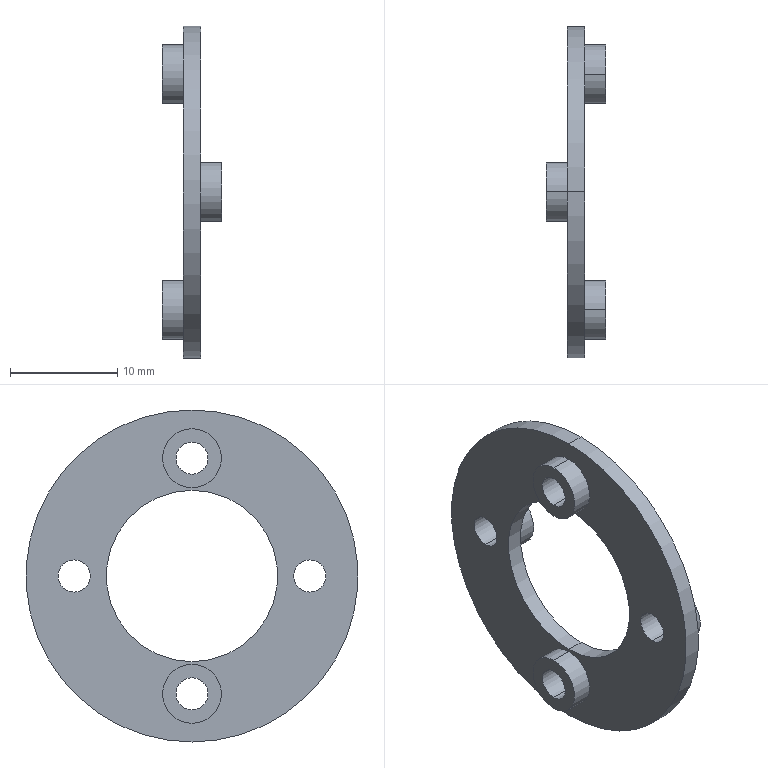Part | SolidWorks | features BaseBody 1 | 1 solid | 26 faces | box 5.6 x 31 x 31 mm | volume 974.208 mm3 | cylinder 20 | plane 6 | commonest cylinder face diameters 3 x8 5.5 x8 16 x2 31 x2
STEP:
#1=CARTESIAN_POINT('',(0.,0.,15.5));
#2=VERTEX_POINT('',#1);
#3=CARTESIAN_POINT('',(0.,0.,-15.5));
#4=VERTEX_POINT('',#3);
#5=CARTESIAN_POINT('',(0.,0.,0.));
#6=DIRECTION('',(1.,0.,0.));
#7=DIRECTION('',(0.,0.,-1.));
#8=AXIS2_PLACEMENT_3D('',#5,#6,#7);
#9=CIRCLE('',#8,15.5);
#10=EDGE_CURVE('',#2,#4,#9,.T.);
#11=ORIENTED_EDGE('',*,*,#10,.T.);
#12=CARTESIAN_POINT('',(1.6,0.,-15.5));
#13=VERTEX_POINT('',#12);
#14=CARTESIAN_POINT('',(1.6,0.,-15.5));
#15=DIRECTION('',(1.,0.,0.));
#16=VECTOR('',#15,1000.);
#17=LINE('',#14,#16);
#18=EDGE_CURVE('',#4,#13,#17,.T.);
#19=ORIENTED_EDGE('',*,*,#18,.T.);
#20=CARTESIAN_POINT('',(1.6,0.,15.5));
#21=VERTEX_POINT('',#20);
#22=CARTESIAN_POINT('',(1.6,0.,0.));
#23=DIRECTION('',(1.,0.,0.));
#24=DIRECTION('',(0.,0.,-1.));
#25=AXIS2_PLACEMENT_3D('',#22,#23,#24);
#26=CIRCLE('',#25,15.5);
#27=EDGE_CURVE('',#21,#13,#26,.T.);
#28=ORIENTED_EDGE('',*,*,#27,.F.);
#29=CARTESIAN_POINT('',(1.6,0.,15.5));
#30=DIRECTION('',(1.,0.,0.));
#31=VECTOR('',#30,1000.);
#32=LINE('',#29,#31);
#33=EDGE_CURVE('',#2,#21,#32,.T.);
#34=ORIENTED_EDGE('',*,*,#33,.F.);
#35=EDGE_LOOP('',(#11,#19,#28,#34));
#36=FACE_OUTER_BOUND('',#35,.T.);
#37=CARTESIAN_POINT('',(1.6,0.,0.));
#38=DIRECTION('',(1.,0.,0.));
#39=DIRECTION('',(0.,0.,1.));
#40=AXIS2_PLACEMENT_3D('',#37,#38,#39);
#41=CYLINDRICAL_SURFACE('',#40,15.5);
#42=ADVANCED_FACE('',(#36),#41,.T.);
#43=CARTESIAN_POINT('',(0.,0.,-8.));
#44=VERTEX_POINT('',#43);
#45=CARTESIAN_POINT('',(0.,0.,8.));
#46=VERTEX_POINT('',#45);
#47=CARTESIAN_POINT('',(0.,0.,0.));
#48=DIRECTION('',(1.,0.,0.));
#49=DIRECTION('',(0.,0.,-1.));
#50=AXIS2_PLACEMENT_3D('',#47,#48,#49);
#51=CIRCLE('',#50,8.);
#52=EDGE_CURVE('',#44,#46,#51,.T.);
#53=ORIENTED_EDGE('',*,*,#52,.F.);
#54=CARTESIAN_POINT('',(1.6,0.,-8.));
#55=VERTEX_POINT('',#54);
#56=CARTESIAN_POINT('',(1.6,0.,-8.));
#57=DIRECTION('',(1.,0.,0.));
#58=VECTOR('',#57,1000.);
#59=LINE('',#56,#58);
#60=EDGE_CURVE('',#44,#55,#59,.T.);
#61=ORIENTED_EDGE('',*,*,#60,.T.);
#62=CARTESIAN_POINT('',(1.6,0.,8.));
#63=VERTEX_POINT('',#62);
#64=CARTESIAN_POINT('',(1.6,0.,0.));
#65=DIRECTION('',(1.,0.,0.));
#66=DIRECTION('',(0.,0.,-1.));
#67=AXIS2_PLACEMENT_3D('',#64,#65,#66);
#68=CIRCLE('',#67,8.);
#69=EDGE_CURVE('',#55,#63,#68,.T.);
#70=ORIENTED_EDGE('',*,*,#69,.T.);
#71=CARTESIAN_POINT('',(1.6,0.,8.));
#72=DIRECTION('',(1.,0.,0.));
#73=VECTOR('',#72,1000.);
#74=LINE('',#71,#73);
#75=EDGE_CURVE('',#46,#63,#74,.T.);
#76=ORIENTED_EDGE('',*,*,#75,.F.);
#77=EDGE_LOOP('',(#53,#61,#70,#76));
#78=FACE_OUTER_BOUND('',#77,.T.);
#79=CARTESIAN_POINT('',(1.6,0.,0.));
#80=DIRECTION('',(1.,0.,0.));
#81=DIRECTION('',(0.,0.,1.));
#82=AXIS2_PLACEMENT_3D('',#79,#80,#81);
#83=CYLINDRICAL_SURFACE('',#82,8.);
#84=ADVANCED_FACE('',(#78),#83,.F.);
#85=CARTESIAN_POINT('',(0.,11.,1.5));
#86=VERTEX_POINT('',#85);
#87=CARTESIAN_POINT('',(0.,11.,-1.5));
#88=VERTEX_POINT('',#87);
#89=CARTESIAN_POINT('',(0.,11.,0.));
#90=DIRECTION('',(-1.,0.,0.));
#91=DIRECTION('',(0.,0.,-1.));
#92=AXIS2_PLACEMENT_3D('',#89,#90,#91);
#93=CIRCLE('',#92,1.5);
#94=EDGE_CURVE('',#86,#88,#93,.T.);
#95=ORIENTED_EDGE('',*,*,#94,.T.);
#96=CARTESIAN_POINT('',(3.6,11.,-1.5));
#97=VERTEX_POINT('',#96);
#98=CARTESIAN_POINT('',(1.6,11.,-1.5));
#99=DIRECTION('',(1.,0.,0.));
#100=VECTOR('',#99,1000.);
#101=LINE('',#98,#100);
#102=EDGE_CURVE('',#88,#97,#101,.T.);
#103=ORIENTED_EDGE('',*,*,#102,.T.);
#104=CARTESIAN_POINT('',(3.6,11.,1.5));
#105=VERTEX_POINT('',#104);
#106=CARTESIAN_POINT('',(3.6,11.,0.));
#107=DIRECTION('',(-1.,0.,0.));
#108=DIRECTION('',(0.,0.,1.));
#109=AXIS2_PLACEMENT_3D('',#106,#107,#108);
#110=CIRCLE('',#109,1.5);
#111=EDGE_CURVE('',#105,#97,#110,.T.);
#112=ORIENTED_EDGE('',*,*,#111,.F.);
#113=CARTESIAN_POINT('',(1.6,11.,1.5));
#114=DIRECTION('',(1.,0.,0.));
#115=VECTOR('',#114,1000.);
#116=LINE('',#113,#115);
#117=EDGE_CURVE('',#86,#105,#116,.T.);
#118=ORIENTED_EDGE('',*,*,#117,.F.);
#119=EDGE_LOOP('',(#95,#103,#112,#118));
#120=FACE_OUTER_BOUND('',#119,.T.);
#121=CARTESIAN_POINT('',(1.6,11.,0.));
#122=DIRECTION('',(1.,0.,0.));
#123=DIRECTION('',(0.,0.,1.));
#124=AXIS2_PLACEMENT_3D('',#121,#122,#123);
#125=CYLINDRICAL_SURFACE('',#124,1.5);
#126=ADVANCED_FACE('',(#120),#125,.F.);
#127=CARTESIAN_POINT('',(-2.,0.,12.5));
#128=VERTEX_POINT('',#127);
#129=CARTESIAN_POINT('',(-2.,0.,9.5));
#130=VERTEX_POINT('',#129);
#131=CARTESIAN_POINT('',(-2.,0.,11.));
#132=DIRECTION('',(-1.,0.,0.));
#133=DIRECTION('',(0.,0.,1.));
#134=AXIS2_PLACEMENT_3D('',#131,#132,#133);
#135=CIRCLE('',#134,1.5);
#136=EDGE_CURVE('',#128,#130,#135,.T.);
#137=ORIENTED_EDGE('',*,*,#136,.T.);
#138=CARTESIAN_POINT('',(1.6,0.,9.5));
#139=VERTEX_POINT('',#138);
#140=CARTESIAN_POINT('',(1.6,0.,9.5));
#141=DIRECTION('',(1.,0.,0.));
#142=VECTOR('',#141,1000.);
#143=LINE('',#140,#142);
#144=EDGE_CURVE('',#130,#139,#143,.T.);
#145=ORIENTED_EDGE('',*,*,#144,.T.);
#146=CARTESIAN_POINT('',(1.6,0.,12.5));
#147=VERTEX_POINT('',#146);
#148=CARTESIAN_POINT('',(1.6,0.,11.));
#149=DIRECTION('',(1.,0.,0.));
#150=DIRECTION('',(0.,0.,-1.));
#151=AXIS2_PLACEMENT_3D('',#148,#149,#150);
#152=CIRCLE('',#151,1.5);
#153=EDGE_CURVE('',#139,#147,#152,.T.);
#154=ORIENTED_EDGE('',*,*,#153,.T.);
#155=CARTESIAN_POINT('',(1.6,0.,12.5));
#156=DIRECTION('',(1.,0.,0.));
#157=VECTOR('',#156,1000.);
#158=LINE('',#155,#157);
#159=EDGE_CURVE('',#128,#147,#158,.T.);
#160=ORIENTED_EDGE('',*,*,#159,.F.);
#161=EDGE_LOOP('',(#137,#145,#154,#160));
#162=FACE_OUTER_BOUND('',#161,.T.);
#163=CARTESIAN_POINT('',(1.6,0.,11.));
#164=DIRECTION('',(1.,0.,0.));
#165=DIRECTION('',(0.,0.,1.));
#166=AXIS2_PLACEMENT_3D('',#163,#164,#165);
#167=CYLINDRICAL_SURFACE('',#166,1.5);
#168=ADVANCED_FACE('',(#162),#167,.F.);
#169=CARTESIAN_POINT('',(0.,-11.,1.5));
#170=VERTEX_POINT('',#169);
#171=CARTESIAN_POINT('',(0.,-11.,-1.5));
#172=VERTEX_POINT('',#171);
#173=CARTESIAN_POINT('',(0.,-11.,0.));
#174=DIRECTION('',(-1.,0.,0.));
#175=DIRECTION('',(0.,0.,-1.));
#176=AXIS2_PLACEMENT_3D('',#173,#174,#175);
#177=CIRCLE('',#176,1.5);
#178=EDGE_CURVE('',#170,#172,#177,.T.);
#179=ORIENTED_EDGE('',*,*,#178,.T.);
#180=CARTESIAN_POINT('',(3.6,-11.,-1.5));
#181=VERTEX_POINT('',#180);
#182=CARTESIAN_POINT('',(1.6,-11.,-1.5));
#183=DIRECTION('',(1.,0.,0.));
#184=VECTOR('',#183,1000.);
#185=LINE('',#182,#184);
#186=EDGE_CURVE('',#172,#181,#185,.T.);
#187=ORIENTED_EDGE('',*,*,#186,.T.);
#188=CARTESIAN_POINT('',(3.6,-11.,1.5));
#189=VERTEX_POINT('',#188);
#190=CARTESIAN_POINT('',(3.6,-11.,0.));
#191=DIRECTION('',(-1.,0.,0.));
#192=DIRECTION('',(0.,0.,1.));
#193=AXIS2_PLACEMENT_3D('',#190,#191,#192);
#194=CIRCLE('',#193,1.5);
#195=EDGE_CURVE('',#189,#181,#194,.T.);
#196=ORIENTED_EDGE('',*,*,#195,.F.);
#197=CARTESIAN_POINT('',(1.6,-11.,1.5));
#198=DIRECTION('',(1.,0.,0.));
#199=VECTOR('',#198,1000.);
#200=LINE('',#197,#199);
#201=EDGE_CURVE('',#170,#189,#200,.T.);
#202=ORIENTED_EDGE('',*,*,#201,.F.);
#203=EDGE_LOOP('',(#179,#187,#196,#202));
#204=FACE_OUTER_BOUND('',#203,.T.);
#205=CARTESIAN_POINT('',(1.6,-11.,0.));
#206=DIRECTION('',(1.,0.,0.));
#207=DIRECTION('',(0.,0.,1.));
#208=AXIS2_PLACEMENT_3D('',#205,#206,#207);
#209=CYLINDRICAL_SURFACE('',#208,1.5);
#210=ADVANCED_FACE('',(#204),#209,.F.);
#211=CARTESIAN_POINT('',(-2.,0.,-9.5));
#212=VERTEX_POINT('',#211);
#213=CARTESIAN_POINT('',(-2.,0.,-12.5));
#214=VERTEX_POINT('',#213);
#215=CARTESIAN_POINT('',(-2.,0.,-11.));
#216=DIRECTION('',(-1.,0.,0.));
#217=DIRECTION('',(0.,0.,1.));
#218=AXIS2_PLACEMENT_3D('',#215,#216,#217);
#219=CIRCLE('',#218,1.5);
#220=EDGE_CURVE('',#212,#214,#219,.T.);
#221=ORIENTED_EDGE('',*,*,#220,.T.);
#222=CARTESIAN_POINT('',(1.6,0.,-12.5));
#223=VERTEX_POINT('',#222);
#224=CARTESIAN_POINT('',(1.6,0.,-12.5));
#225=DIRECTION('',(1.,0.,0.));
#226=VECTOR('',#225,1000.);
#227=LINE('',#224,#226);
#228=EDGE_CURVE('',#214,#223,#227,.T.);
#229=ORIENTED_EDGE('',*,*,#228,.T.);
#230=CARTESIAN_POINT('',(1.6,0.,-9.5));
#231=VERTEX_POINT('',#230);
#232=CARTESIAN_POINT('',(1.6,0.,-11.));
#233=DIRECTION('',(1.,0.,0.));
#234=DIRECTION('',(0.,0.,-1.));
#235=AXIS2_PLACEMENT_3D('',#232,#233,#234);
#236=CIRCLE('',#235,1.5);
#237=EDGE_CURVE('',#223,#231,#236,.T.);
#238=ORIENTED_EDGE('',*,*,#237,.T.);
#239=CARTESIAN_POINT('',(1.6,0.,-9.5));
#240=DIRECTION('',(1.,0.,0.));
#241=VECTOR('',#240,1000.);
#242=LINE('',#239,#241);
#243=EDGE_CURVE('',#212,#231,#242,.T.);
#244=ORIENTED_EDGE('',*,*,#243,.F.);
#245=EDGE_LOOP('',(#221,#229,#238,#244));
#246=FACE_OUTER_BOUND('',#245,.T.);
#247=CARTESIAN_POINT('',(1.6,0.,-11.));
#248=DIRECTION('',(1.,0.,0.));
#249=DIRECTION('',(0.,0.,1.));
#250=AXIS2_PLACEMENT_3D('',#247,#248,#249);
#251=CYLINDRICAL_SURFACE('',#250,1.5);
#252=ADVANCED_FACE('',(#246),#251,.F.);
#253=CARTESIAN_POINT('',(1.6,11.,2.75));
#254=VERTEX_POINT('',#253);
#255=CARTESIAN_POINT('',(1.6,11.,-2.75));
#256=VERTEX_POINT('',#255);
#257=CARTESIAN_POINT('',(1.6,11.,0.));
#258=DIRECTION('',(1.,0.,0.));
#259=DIRECTION('',(0.,0.,-1.));
#260=AXIS2_PLACEMENT_3D('',#257,#258,#259);
#261=CIRCLE('',#260,2.75);
#262=EDGE_CURVE('',#254,#256,#261,.T.);
#263=ORIENTED_EDGE('',*,*,#262,.T.);
#264=CARTESIAN_POINT('',(3.6,11.,-2.75));
#265=VERTEX_POINT('',#264);
#266=CARTESIAN_POINT('',(1.6,11.,-2.75));
#267=DIRECTION('',(1.,0.,0.));
#268=VECTOR('',#267,1000.);
#269=LINE('',#266,#268);
#270=EDGE_CURVE('',#256,#265,#269,.T.);
#271=ORIENTED_EDGE('',*,*,#270,.T.);
#272=CARTESIAN_POINT('',(3.6,11.,2.75));
#273=VERTEX_POINT('',#272);
#274=CARTESIAN_POINT('',(3.6,11.,0.));
#275=DIRECTION('',(-1.,0.,0.));
#276=DIRECTION('',(0.,0.,1.));
#277=AXIS2_PLACEMENT_3D('',#274,#275,#276);
#278=CIRCLE('',#277,2.75);
#279=EDGE_CURVE('',#265,#273,#278,.T.);
#280=ORIENTED_EDGE('',*,*,#279,.T.);
#281=CARTESIAN_POINT('',(1.6,11.,2.75));
#282=DIRECTION('',(1.,0.,0.));
#283=VECTOR('',#282,1000.);
#284=LINE('',#281,#283);
#285=EDGE_CURVE('',#254,#273,#284,.T.);
#286=ORIENTED_EDGE('',*,*,#285,.F.);
#287=EDGE_LOOP('',(#263,#271,#280,#286));
#288=FACE_OUTER_BOUND('',#287,.T.);
#289=CARTESIAN_POINT('',(1.6,11.,0.));
#290=DIRECTION('',(1.,0.,0.));
#291=DIRECTION('',(0.,0.,1.));
#292=AXIS2_PLACEMENT_3D('',#289,#290,#291);
#293=CYLINDRICAL_SURFACE('',#292,2.75);
#294=ADVANCED_FACE('',(#288),#293,.T.);
#295=CARTESIAN_POINT('',(1.6,-11.,2.75));
#296=VERTEX_POINT('',#295);
#297=CARTESIAN_POINT('',(1.6,-11.,-2.75));
#298=VERTEX_POINT('',#297);
#299=CARTESIAN_POINT('',(1.6,-11.,0.));
#300=DIRECTION('',(1.,0.,0.));
#301=DIRECTION('',(0.,0.,-1.));
#302=AXIS2_PLACEMENT_3D('',#299,#300,#301);
#303=CIRCLE('',#302,2.75);
#304=EDGE_CURVE('',#296,#298,#303,.T.);
#305=ORIENTED_EDGE('',*,*,#304,.T.);
#306=CARTESIAN_POINT('',(3.6,-11.,-2.75));
#307=VERTEX_POINT('',#306);
#308=CARTESIAN_POINT('',(1.6,-11.,-2.75));
#309=DIRECTION('',(1.,0.,0.));
#310=VECTOR('',#309,1000.);
#311=LINE('',#308,#310);
#312=EDGE_CURVE('',#298,#307,#311,.T.);
#313=ORIENTED_EDGE('',*,*,#312,.T.);
#314=CARTESIAN_POINT('',(3.6,-11.,2.75));
#315=VERTEX_POINT('',#314);
#316=CARTESIAN_POINT('',(3.6,-11.,0.));
#317=DIRECTION('',(-1.,0.,0.));
#318=DIRECTION('',(0.,0.,1.));
#319=AXIS2_PLACEMENT_3D('',#316,#317,#318);
#320=CIRCLE('',#319,2.75);
#321=EDGE_CURVE('',#307,#315,#320,.T.);
#322=ORIENTED_EDGE('',*,*,#321,.T.);
#323=CARTESIAN_POINT('',(1.6,-11.,2.75));
#324=DIRECTION('',(1.,0.,0.));
#325=VECTOR('',#324,1000.);
#326=LINE('',#323,#325);
#327=EDGE_CURVE('',#296,#315,#326,.T.);
#328=ORIENTED_EDGE('',*,*,#327,.F.);
#329=EDGE_LOOP('',(#305,#313,#322,#328));
#330=FACE_OUTER_BOUND('',#329,.T.);
#331=CARTESIAN_POINT('',(1.6,-11.,0.));
#332=DIRECTION('',(1.,0.,0.));
#333=DIRECTION('',(0.,0.,1.));
#334=AXIS2_PLACEMENT_3D('',#331,#332,#333);
#335=CYLINDRICAL_SURFACE('',#334,2.75);
#336=ADVANCED_FACE('',(#330),#335,.T.);
#337=CARTESIAN_POINT('',(-2.,0.,-13.75));
#338=VERTEX_POINT('',#337);
#339=CARTESIAN_POINT('',(-2.,0.,-8.25));
#340=VERTEX_POINT('',#339);
#341=CARTESIAN_POINT('',(-2.,0.,-11.));
#342=DIRECTION('',(-1.,0.,0.));
#343=DIRECTION('',(0.,0.,1.));
#344=AXIS2_PLACEMENT_3D('',#341,#342,#343);
#345=CIRCLE('',#344,2.75);
#346=EDGE_CURVE('',#338,#340,#345,.T.);
#347=ORIENTED_EDGE('',*,*,#346,.F.);
#348=CARTESIAN_POINT('',(0.,0.,-13.75));
#349=VERTEX_POINT('',#348);
#350=CARTESIAN_POINT('',(-2.,0.,-13.75));
#351=DIRECTION('',(1.,0.,0.));
#352=VECTOR('',#351,1000.);
#353=LINE('',#350,#352);
#354=EDGE_CURVE('',#338,#349,#353,.T.);
#355=ORIENTED_EDGE('',*,*,#354,.T.);
#356=CARTESIAN_POINT('',(0.,0.,-8.25));
#357=VERTEX_POINT('',#356);
#358=CARTESIAN_POINT('',(0.,0.,-11.));
#359=DIRECTION('',(-1.,0.,0.));
#360=DIRECTION('',(0.,0.,1.));
#361=AXIS2_PLACEMENT_3D('',#358,#359,#360);
#362=CIRCLE('',#361,2.75);
#363=EDGE_CURVE('',#349,#357,#362,.T.);
#364=ORIENTED_EDGE('',*,*,#363,.T.);
#365=CARTESIAN_POINT('',(-2.,0.,-8.25));
#366=DIRECTION('',(1.,0.,0.));
#367=VECTOR('',#366,1000.);
#368=LINE('',#365,#367);
#369=EDGE_CURVE('',#340,#357,#368,.T.);
#370=ORIENTED_EDGE('',*,*,#369,.F.);
#371=EDGE_LOOP('',(#347,#355,#364,#370));
#372=FACE_OUTER_BOUND('',#371,.T.);
#373=CARTESIAN_POINT('',(-2.,0.,-11.));
#374=DIRECTION('',(1.,0.,0.));
#375=DIRECTION('',(0.,0.,1.));
#376=AXIS2_PLACEMENT_3D('',#373,#374,#375);
#377=CYLINDRICAL_SURFACE('',#376,2.75);
#378=ADVANCED_FACE('',(#372),#377,.T.);
#379=CARTESIAN_POINT('',(-2.,0.,8.25));
#380=VERTEX_POINT('',#379);
#381=CARTESIAN_POINT('',(-2.,0.,13.75));
#382=VERTEX_POINT('',#381);
#383=CARTESIAN_POINT('',(-2.,0.,11.));
#384=DIRECTION('',(-1.,0.,0.));
#385=DIRECTION('',(0.,0.,1.));
#386=AXIS2_PLACEMENT_3D('',#383,#384,#385);
#387=CIRCLE('',#386,2.75);
#388=EDGE_CURVE('',#380,#382,#387,.T.);
#389=ORIENTED_EDGE('',*,*,#388,.F.);
#390=CARTESIAN_POINT('',(0.,0.,8.25));
#391=VERTEX_POINT('',#390);
#392=CARTESIAN_POINT('',(-2.,0.,8.25));
#393=DIRECTION('',(1.,0.,0.));
#394=VECTOR('',#393,1000.);
#395=LINE('',#392,#394);
#396=EDGE_CURVE('',#380,#391,#395,.T.);
#397=ORIENTED_EDGE('',*,*,#396,.T.);
#398=CARTESIAN_POINT('',(0.,0.,13.75));
#399=VERTEX_POINT('',#398);
#400=CARTESIAN_POINT('',(0.,0.,11.));
#401=DIRECTION('',(-1.,0.,0.));
#402=DIRECTION('',(0.,0.,1.));
#403=AXIS2_PLACEMENT_3D('',#400,#401,#402);
#404=CIRCLE('',#403,2.75);
#405=EDGE_CURVE('',#391,#399,#404,.T.);
#406=ORIENTED_EDGE('',*,*,#405,.T.);
#407=CARTESIAN_POINT('',(-2.,0.,13.75));
#408=DIRECTION('',(1.,0.,0.));
#409=VECTOR('',#408,1000.);
#410=LINE('',#407,#409);
#411=EDGE_CURVE('',#382,#399,#410,.T.);
#412=ORIENTED_EDGE('',*,*,#411,.F.);
#413=EDGE_LOOP('',(#389,#397,#406,#412));
#414=FACE_OUTER_BOUND('',#413,.T.);
#415=CARTESIAN_POINT('',(-2.,0.,11.));
#416=DIRECTION('',(1.,0.,0.));
#417=DIRECTION('',(0.,0.,1.));
#418=AXIS2_PLACEMENT_3D('',#415,#416,#417);
#419=CYLINDRICAL_SURFACE('',#418,2.75);
#420=ADVANCED_FACE('',(#414),#419,.T.);
#421=ORIENTED_EDGE('',*,*,#396,.F.);
#422=CARTESIAN_POINT('',(-2.,0.,11.));
#423=DIRECTION('',(-1.,0.,0.));
#424=DIRECTION('',(0.,0.,1.));
#425=AXIS2_PLACEMENT_3D('',#422,#423,#424);
#426=CIRCLE('',#425,2.75);
#427=EDGE_CURVE('',#382,#380,#426,.T.);
#428=ORIENTED_EDGE('',*,*,#427,.F.);
#429=ORIENTED_EDGE('',*,*,#411,.T.);
#430=CARTESIAN_POINT('',(0.,0.,11.));
#431=DIRECTION('',(-1.,0.,0.));
#432=DIRECTION('',(0.,0.,1.));
#433=AXIS2_PLACEMENT_3D('',#430,#431,#432);
#434=CIRCLE('',#433,2.75);
#435=EDGE_CURVE('',#399,#391,#434,.T.);
#436=ORIENTED_EDGE('',*,*,#435,.T.);
#437=EDGE_LOOP('',(#421,#428,#429,#436));
#438=FACE_OUTER_BOUND('',#437,.T.);
#439=CARTESIAN_POINT('',(-2.,0.,11.));
#440=DIRECTION('',(1.,0.,0.));
#441=DIRECTION('',(0.,0.,1.));
#442=AXIS2_PLACEMENT_3D('',#439,#440,#441);
#443=CYLINDRICAL_SURFACE('',#442,2.75);
#444=ADVANCED_FACE('',(#438),#443,.T.);
#445=ORIENTED_EDGE('',*,*,#136,.F.);
#446=CARTESIAN_POINT('',(-2.,0.,11.));
#447=DIRECTION('',(-1.,0.,0.));
#448=DIRECTION('',(0.,0.,1.));
#449=AXIS2_PLACEMENT_3D('',#446,#447,#448);
#450=CIRCLE('',#449,1.5);
#451=EDGE_CURVE('',#130,#128,#450,.T.);
#452=ORIENTED_EDGE('',*,*,#451,.F.);
#453=EDGE_LOOP('',(#445,#452));
#454=FACE_BOUND('',#453,.T.);
#455=ORIENTED_EDGE('',*,*,#427,.T.);
#456=ORIENTED_EDGE('',*,*,#388,.T.);
#457=EDGE_LOOP('',(#455,#456));
#458=FACE_OUTER_BOUND('',#457,.T.);
#459=CARTESIAN_POINT('',(-2.,0.,12.5));
#460=DIRECTION('',(-1.,0.,0.));
#461=DIRECTION('',(0.,0.,1.));
#462=AXIS2_PLACEMENT_3D('',#459,#460,#461);
#463=PLANE('',#462);
#464=ADVANCED_FACE('',(#454,#458),#463,.T.);
#465=ORIENTED_EDGE('',*,*,#354,.F.);
#466=CARTESIAN_POINT('',(-2.,0.,-11.));
#467=DIRECTION('',(-1.,0.,0.));
#468=DIRECTION('',(0.,0.,1.));
#469=AXIS2_PLACEMENT_3D('',#466,#467,#468);
#470=CIRCLE('',#469,2.75);
#471=EDGE_CURVE('',#340,#338,#470,.T.);
#472=ORIENTED_EDGE('',*,*,#471,.F.);
#473=ORIENTED_EDGE('',*,*,#369,.T.);
#474=CARTESIAN_POINT('',(0.,0.,-11.));
#475=DIRECTION('',(-1.,0.,0.));
#476=DIRECTION('',(0.,0.,1.));
#477=AXIS2_PLACEMENT_3D('',#474,#475,#476);
#478=CIRCLE('',#477,2.75);
#479=EDGE_CURVE('',#357,#349,#478,.T.);
#480=ORIENTED_EDGE('',*,*,#479,.T.);
#481=EDGE_LOOP('',(#465,#472,#473,#480));
#482=FACE_OUTER_BOUND('',#481,.T.);
#483=CARTESIAN_POINT('',(-2.,0.,-11.));
#484=DIRECTION('',(1.,0.,0.));
#485=DIRECTION('',(0.,0.,1.));
#486=AXIS2_PLACEMENT_3D('',#483,#484,#485);
#487=CYLINDRICAL_SURFACE('',#486,2.75);
#488=ADVANCED_FACE('',(#482),#487,.T.);
#489=ORIENTED_EDGE('',*,*,#220,.F.);
#490=CARTESIAN_POINT('',(-2.,0.,-11.));
#491=DIRECTION('',(-1.,0.,0.));
#492=DIRECTION('',(0.,0.,1.));
#493=AXIS2_PLACEMENT_3D('',#490,#491,#492);
#494=CIRCLE('',#493,1.5);
#495=EDGE_CURVE('',#214,#212,#494,.T.);
#496=ORIENTED_EDGE('',*,*,#495,.F.);
#497=EDGE_LOOP('',(#489,#496));
#498=FACE_BOUND('',#497,.T.);
#499=ORIENTED_EDGE('',*,*,#471,.T.);
#500=ORIENTED_EDGE('',*,*,#346,.T.);
#501=EDGE_LOOP('',(#499,#500));
#502=FACE_OUTER_BOUND('',#501,.T.);
#503=CARTESIAN_POINT('',(-2.,0.,-9.5));
#504=DIRECTION('',(-1.,0.,0.));
#505=DIRECTION('',(0.,0.,1.));
#506=AXIS2_PLACEMENT_3D('',#503,#504,#505);
#507=PLANE('',#506);
#508=ADVANCED_FACE('',(#498,#502),#507,.T.);
#509=ORIENTED_EDGE('',*,*,#195,.T.);
#510=CARTESIAN_POINT('',(3.6,-11.,0.));
#511=DIRECTION('',(-1.,0.,0.));
#512=DIRECTION('',(0.,0.,1.));
#513=AXIS2_PLACEMENT_3D('',#510,#511,#512);
#514=CIRCLE('',#513,1.5);
#515=EDGE_CURVE('',#181,#189,#514,.T.);
#516=ORIENTED_EDGE('',*,*,#515,.T.);
#517=EDGE_LOOP('',(#509,#516));
#518=FACE_BOUND('',#517,.T.);
#519=CARTESIAN_POINT('',(3.6,-11.,0.));
#520=DIRECTION('',(-1.,0.,0.));
#521=DIRECTION('',(0.,0.,1.));
#522=AXIS2_PLACEMENT_3D('',#519,#520,#521);
#523=CIRCLE('',#522,2.75);
#524=EDGE_CURVE('',#315,#307,#523,.T.);
#525=ORIENTED_EDGE('',*,*,#524,.F.);
#526=ORIENTED_EDGE('',*,*,#321,.F.);
#527=EDGE_LOOP('',(#525,#526));
#528=FACE_OUTER_BOUND('',#527,.T.);
#529=CARTESIAN_POINT('',(3.6,-13.75,0.));
#530=DIRECTION('',(1.,0.,0.));
#531=DIRECTION('',(0.,1.,0.));
#532=AXIS2_PLACEMENT_3D('',#529,#530,#531);
#533=PLANE('',#532);
#534=ADVANCED_FACE('',(#518,#528),#533,.T.);
#535=ORIENTED_EDGE('',*,*,#312,.F.);
#536=CARTESIAN_POINT('',(1.6,-11.,0.));
#537=DIRECTION('',(1.,0.,0.));
#538=DIRECTION('',(0.,0.,-1.));
#539=AXIS2_PLACEMENT_3D('',#536,#537,#538);
#540=CIRCLE('',#539,2.75);
#541=EDGE_CURVE('',#298,#296,#540,.T.);
#542=ORIENTED_EDGE('',*,*,#541,.T.);
#543=ORIENTED_EDGE('',*,*,#327,.T.);
#544=ORIENTED_EDGE('',*,*,#524,.T.);
#545=EDGE_LOOP('',(#535,#542,#543,#544));
#546=FACE_OUTER_BOUND('',#545,.T.);
#547=CARTESIAN_POINT('',(1.6,-11.,0.));
#548=DIRECTION('',(1.,0.,0.));
#549=DIRECTION('',(0.,0.,1.));
#550=AXIS2_PLACEMENT_3D('',#547,#548,#549);
#551=CYLINDRICAL_SURFACE('',#550,2.75);
#552=ADVANCED_FACE('',(#546),#551,.T.);
#553=ORIENTED_EDGE('',*,*,#111,.T.);
#554=CARTESIAN_POINT('',(3.6,11.,0.));
#555=DIRECTION('',(-1.,0.,0.));
#556=DIRECTION('',(0.,0.,1.));
#557=AXIS2_PLACEMENT_3D('',#554,#555,#556);
#558=CIRCLE('',#557,1.5);
#559=EDGE_CURVE('',#97,#105,#558,.T.);
#560=ORIENTED_EDGE('',*,*,#559,.T.);
#561=EDGE_LOOP('',(#553,#560));
#562=FACE_BOUND('',#561,.T.);
#563=CARTESIAN_POINT('',(3.6,11.,0.));
#564=DIRECTION('',(-1.,0.,0.));
#565=DIRECTION('',(0.,0.,1.));
#566=AXIS2_PLACEMENT_3D('',#563,#564,#565);
#567=CIRCLE('',#566,2.75);
#568=EDGE_CURVE('',#273,#265,#567,.T.);
#569=ORIENTED_EDGE('',*,*,#568,.F.);
#570=ORIENTED_EDGE('',*,*,#279,.F.);
#571=EDGE_LOOP('',(#569,#570));
#572=FACE_OUTER_BOUND('',#571,.T.);
#573=CARTESIAN_POINT('',(3.6,8.25,0.));
#574=DIRECTION('',(1.,0.,0.));
#575=DIRECTION('',(0.,1.,0.));
#576=AXIS2_PLACEMENT_3D('',#573,#574,#575);
#577=PLANE('',#576);
#578=ADVANCED_FACE('',(#562,#572),#577,.T.);
#579=ORIENTED_EDGE('',*,*,#270,.F.);
#580=CARTESIAN_POINT('',(1.6,11.,0.));
#581=DIRECTION('',(1.,0.,0.));
#582=DIRECTION('',(0.,0.,-1.));
#583=AXIS2_PLACEMENT_3D('',#580,#581,#582);
#584=CIRCLE('',#583,2.75);
#585=EDGE_CURVE('',#256,#254,#584,.T.);
#586=ORIENTED_EDGE('',*,*,#585,.T.);
#587=ORIENTED_EDGE('',*,*,#285,.T.);
#588=ORIENTED_EDGE('',*,*,#568,.T.);
#589=EDGE_LOOP('',(#579,#586,#587,#588));
#590=FACE_OUTER_BOUND('',#589,.T.);
#591=CARTESIAN_POINT('',(1.6,11.,0.));
#592=DIRECTION('',(1.,0.,0.));
#593=DIRECTION('',(0.,0.,1.));
#594=AXIS2_PLACEMENT_3D('',#591,#592,#593);
#595=CYLINDRICAL_SURFACE('',#594,2.75);
#596=ADVANCED_FACE('',(#590),#595,.T.);
#597=ORIENTED_EDGE('',*,*,#228,.F.);
#598=ORIENTED_EDGE('',*,*,#495,.T.);
#599=ORIENTED_EDGE('',*,*,#243,.T.);
#600=CARTESIAN_POINT('',(1.6,0.,-11.));
#601=DIRECTION('',(1.,0.,0.));
#602=DIRECTION('',(0.,0.,-1.));
#603=AXIS2_PLACEMENT_3D('',#600,#601,#602);
#604=CIRCLE('',#603,1.5);
#605=EDGE_CURVE('',#231,#223,#604,.T.);
#606=ORIENTED_EDGE('',*,*,#605,.T.);
#607=EDGE_LOOP('',(#597,#598,#599,#606));
#608=FACE_OUTER_BOUND('',#607,.T.);
#609=CARTESIAN_POINT('',(1.6,0.,-11.));
#610=DIRECTION('',(1.,0.,0.));
#611=DIRECTION('',(0.,0.,1.));
#612=AXIS2_PLACEMENT_3D('',#609,#610,#611);
#613=CYLINDRICAL_SURFACE('',#612,1.5);
#614=ADVANCED_FACE('',(#608),#613,.F.);
#615=ORIENTED_EDGE('',*,*,#186,.F.);
#616=CARTESIAN_POINT('',(0.,-11.,0.));
#617=DIRECTION('',(-1.,0.,0.));
#618=DIRECTION('',(0.,0.,-1.));
#619=AXIS2_PLACEMENT_3D('',#616,#617,#618);
#620=CIRCLE('',#619,1.5);
#621=EDGE_CURVE('',#172,#170,#620,.T.);
#622=ORIENTED_EDGE('',*,*,#621,.T.);
#623=ORIENTED_EDGE('',*,*,#201,.T.);
#624=ORIENTED_EDGE('',*,*,#515,.F.);
#625=EDGE_LOOP('',(#615,#622,#623,#624));
#626=FACE_OUTER_BOUND('',#625,.T.);
#627=CARTESIAN_POINT('',(1.6,-11.,0.));
#628=DIRECTION('',(1.,0.,0.));
#629=DIRECTION('',(0.,0.,1.));
#630=AXIS2_PLACEMENT_3D('',#627,#628,#629);
#631=CYLINDRICAL_SURFACE('',#630,1.5);
#632=ADVANCED_FACE('',(#626),#631,.F.);
#633=ORIENTED_EDGE('',*,*,#144,.F.);
#634=ORIENTED_EDGE('',*,*,#451,.T.);
#635=ORIENTED_EDGE('',*,*,#159,.T.);
#636=CARTESIAN_POINT('',(1.6,0.,11.));
#637=DIRECTION('',(1.,0.,0.));
#638=DIRECTION('',(0.,0.,-1.));
#639=AXIS2_PLACEMENT_3D('',#636,#637,#638);
#640=CIRCLE('',#639,1.5);
#641=EDGE_CURVE('',#147,#139,#640,.T.);
#642=ORIENTED_EDGE('',*,*,#641,.T.);
#643=EDGE_LOOP('',(#633,#634,#635,#642));
#644=FACE_OUTER_BOUND('',#643,.T.);
#645=CARTESIAN_POINT('',(1.6,0.,11.));
#646=DIRECTION('',(1.,0.,0.));
#647=DIRECTION('',(0.,0.,1.));
#648=AXIS2_PLACEMENT_3D('',#645,#646,#647);
#649=CYLINDRICAL_SURFACE('',#648,1.5);
#650=ADVANCED_FACE('',(#644),#649,.F.);
#651=ORIENTED_EDGE('',*,*,#102,.F.);
#652=CARTESIAN_POINT('',(0.,11.,0.));
#653=DIRECTION('',(-1.,0.,0.));
#654=DIRECTION('',(0.,0.,-1.));
#655=AXIS2_PLACEMENT_3D('',#652,#653,#654);
#656=CIRCLE('',#655,1.5);
#657=EDGE_CURVE('',#88,#86,#656,.T.);
#658=ORIENTED_EDGE('',*,*,#657,.T.);
#659=ORIENTED_EDGE('',*,*,#117,.T.);
#660=ORIENTED_EDGE('',*,*,#559,.F.);
#661=EDGE_LOOP('',(#651,#658,#659,#660));
#662=FACE_OUTER_BOUND('',#661,.T.);
#663=CARTESIAN_POINT('',(1.6,11.,0.));
#664=DIRECTION('',(1.,0.,0.));
#665=DIRECTION('',(0.,0.,1.));
#666=AXIS2_PLACEMENT_3D('',#663,#664,#665);
#667=CYLINDRICAL_SURFACE('',#666,1.5);
#668=ADVANCED_FACE('',(#662),#667,.F.);
#669=ORIENTED_EDGE('',*,*,#60,.F.);
#670=CARTESIAN_POINT('',(0.,0.,0.));
#671=DIRECTION('',(1.,0.,0.));
#672=DIRECTION('',(0.,0.,-1.));
#673=AXIS2_PLACEMENT_3D('',#670,#671,#672);
#674=CIRCLE('',#673,8.);
#675=EDGE_CURVE('',#46,#44,#674,.T.);
#676=ORIENTED_EDGE('',*,*,#675,.F.);
#677=ORIENTED_EDGE('',*,*,#75,.T.);
#678=CARTESIAN_POINT('',(1.6,0.,0.));
#679=DIRECTION('',(1.,0.,0.));
#680=DIRECTION('',(0.,0.,-1.));
#681=AXIS2_PLACEMENT_3D('',#678,#679,#680);
#682=CIRCLE('',#681,8.);
#683=EDGE_CURVE('',#63,#55,#682,.T.);
#684=ORIENTED_EDGE('',*,*,#683,.T.);
#685=EDGE_LOOP('',(#669,#676,#677,#684));
#686=FACE_OUTER_BOUND('',#685,.T.);
#687=CARTESIAN_POINT('',(1.6,0.,0.));
#688=DIRECTION('',(1.,0.,0.));
#689=DIRECTION('',(0.,0.,1.));
#690=AXIS2_PLACEMENT_3D('',#687,#688,#689);
#691=CYLINDRICAL_SURFACE('',#690,8.);
#692=ADVANCED_FACE('',(#686),#691,.F.);
#693=ORIENTED_EDGE('',*,*,#683,.F.);
#694=ORIENTED_EDGE('',*,*,#69,.F.);
#695=EDGE_LOOP('',(#693,#694));
#696=FACE_BOUND('',#695,.T.);
#697=ORIENTED_EDGE('',*,*,#641,.F.);
#698=ORIENTED_EDGE('',*,*,#153,.F.);
#699=EDGE_LOOP('',(#697,#698));
#700=FACE_BOUND('',#699,.T.);
#701=ORIENTED_EDGE('',*,*,#605,.F.);
#702=ORIENTED_EDGE('',*,*,#237,.F.);
#703=EDGE_LOOP('',(#701,#702));
#704=FACE_BOUND('',#703,.T.);
#705=ORIENTED_EDGE('',*,*,#262,.F.);
#706=ORIENTED_EDGE('',*,*,#585,.F.);
#707=EDGE_LOOP('',(#705,#706));
#708=FACE_BOUND('',#707,.T.);
#709=ORIENTED_EDGE('',*,*,#304,.F.);
#710=ORIENTED_EDGE('',*,*,#541,.F.);
#711=EDGE_LOOP('',(#709,#710));
#712=FACE_BOUND('',#711,.T.);
#713=ORIENTED_EDGE('',*,*,#27,.T.);
#714=CARTESIAN_POINT('',(1.6,0.,0.));
#715=DIRECTION('',(1.,0.,0.));
#716=DIRECTION('',(0.,0.,-1.));
#717=AXIS2_PLACEMENT_3D('',#714,#715,#716);
#718=CIRCLE('',#717,15.5);
#719=EDGE_CURVE('',#13,#21,#718,.T.);
#720=ORIENTED_EDGE('',*,*,#719,.T.);
#721=EDGE_LOOP('',(#713,#720));
#722=FACE_OUTER_BOUND('',#721,.T.);
#723=CARTESIAN_POINT('',(1.6,0.,0.));
#724=DIRECTION('',(1.,0.,0.));
#725=DIRECTION('',(0.,1.,0.));
#726=AXIS2_PLACEMENT_3D('',#723,#724,#725);
#727=PLANE('',#726);
#728=ADVANCED_FACE('',(#696,#700,#704,#708,#712,#722),#727,.T.);
#729=ORIENTED_EDGE('',*,*,#18,.F.);
#730=CARTESIAN_POINT('',(0.,0.,0.));
#731=DIRECTION('',(1.,0.,0.));
#732=DIRECTION('',(0.,0.,-1.));
#733=AXIS2_PLACEMENT_3D('',#730,#731,#732);
#734=CIRCLE('',#733,15.5);
#735=EDGE_CURVE('',#4,#2,#734,.T.);
#736=ORIENTED_EDGE('',*,*,#735,.T.);
#737=ORIENTED_EDGE('',*,*,#33,.T.);
#738=ORIENTED_EDGE('',*,*,#719,.F.);
#739=EDGE_LOOP('',(#729,#736,#737,#738));
#740=FACE_OUTER_BOUND('',#739,.T.);
#741=CARTESIAN_POINT('',(1.6,0.,0.));
#742=DIRECTION('',(1.,0.,0.));
#743=DIRECTION('',(0.,0.,1.));
#744=AXIS2_PLACEMENT_3D('',#741,#742,#743);
#745=CYLINDRICAL_SURFACE('',#744,15.5);
#746=ADVANCED_FACE('',(#740),#745,.T.);
#747=ORIENTED_EDGE('',*,*,#675,.T.);
#748=ORIENTED_EDGE('',*,*,#52,.T.);
#749=EDGE_LOOP('',(#747,#748));
#750=FACE_BOUND('',#749,.T.);
#751=ORIENTED_EDGE('',*,*,#94,.F.);
#752=ORIENTED_EDGE('',*,*,#657,.F.);
#753=EDGE_LOOP('',(#751,#752));
#754=FACE_BOUND('',#753,.T.);
#755=ORIENTED_EDGE('',*,*,#178,.F.);
#756=ORIENTED_EDGE('',*,*,#621,.F.);
#757=EDGE_LOOP('',(#755,#756));
#758=FACE_BOUND('',#757,.T.);
#759=ORIENTED_EDGE('',*,*,#479,.F.);
#760=ORIENTED_EDGE('',*,*,#363,.F.);
#761=EDGE_LOOP('',(#759,#760));
#762=FACE_BOUND('',#761,.T.);
#763=ORIENTED_EDGE('',*,*,#435,.F.);
#764=ORIENTED_EDGE('',*,*,#405,.F.);
#765=EDGE_LOOP('',(#763,#764));
#766=FACE_BOUND('',#765,.T.);
#767=ORIENTED_EDGE('',*,*,#10,.F.);
#768=ORIENTED_EDGE('',*,*,#735,.F.);
#769=EDGE_LOOP('',(#767,#768));
#770=FACE_OUTER_BOUND('',#769,.T.);
#771=CARTESIAN_POINT('',(0.,0.,0.));
#772=DIRECTION('',(1.,0.,0.));
#773=DIRECTION('',(0.,1.,0.));
#774=AXIS2_PLACEMENT_3D('',#771,#772,#773);
#775=PLANE('',#774);
#776=ADVANCED_FACE('',(#750,#754,#758,#762,#766,#770),#775,.F.);
#777=CLOSED_SHELL('',(#42,#84,#126,#168,#210,#252,#294,#336,#378,#420,#444,#464,#488,#508,#534,#552,#578,#596,#614,#632,#650,#668,#692,#728,#746,#776));
#778=MANIFOLD_SOLID_BREP('',#777);
#779=CARTESIAN_POINT('',(0.,0.,0.));
#780=DIRECTION('',(0.,0.,1.));
#781=DIRECTION('',(1.,0.,0.));
#782=AXIS2_PLACEMENT_3D('',#779,#780,#781);
#783=(LENGTH_UNIT()NAMED_UNIT(*)SI_UNIT(.MILLI.,.METRE.));
#784=UNCERTAINTY_MEASURE_WITH_UNIT(LENGTH_MEASURE(0.00001),#783,'','');
#785=(NAMED_UNIT(*)PLANE_ANGLE_UNIT()SI_UNIT($,.RADIAN.));
#786=(NAMED_UNIT(*)SI_UNIT($,.STERADIAN.)SOLID_ANGLE_UNIT());
#787=(GEOMETRIC_REPRESENTATION_CONTEXT(3)GLOBAL_UNCERTAINTY_ASSIGNED_CONTEXT((#784))GLOBAL_UNIT_ASSIGNED_CONTEXT((#783,#785,#786))REPRESENTATION_CONTEXT('',''));
#788=ADVANCED_BREP_SHAPE_REPRESENTATION('',(#778,#782),#787);